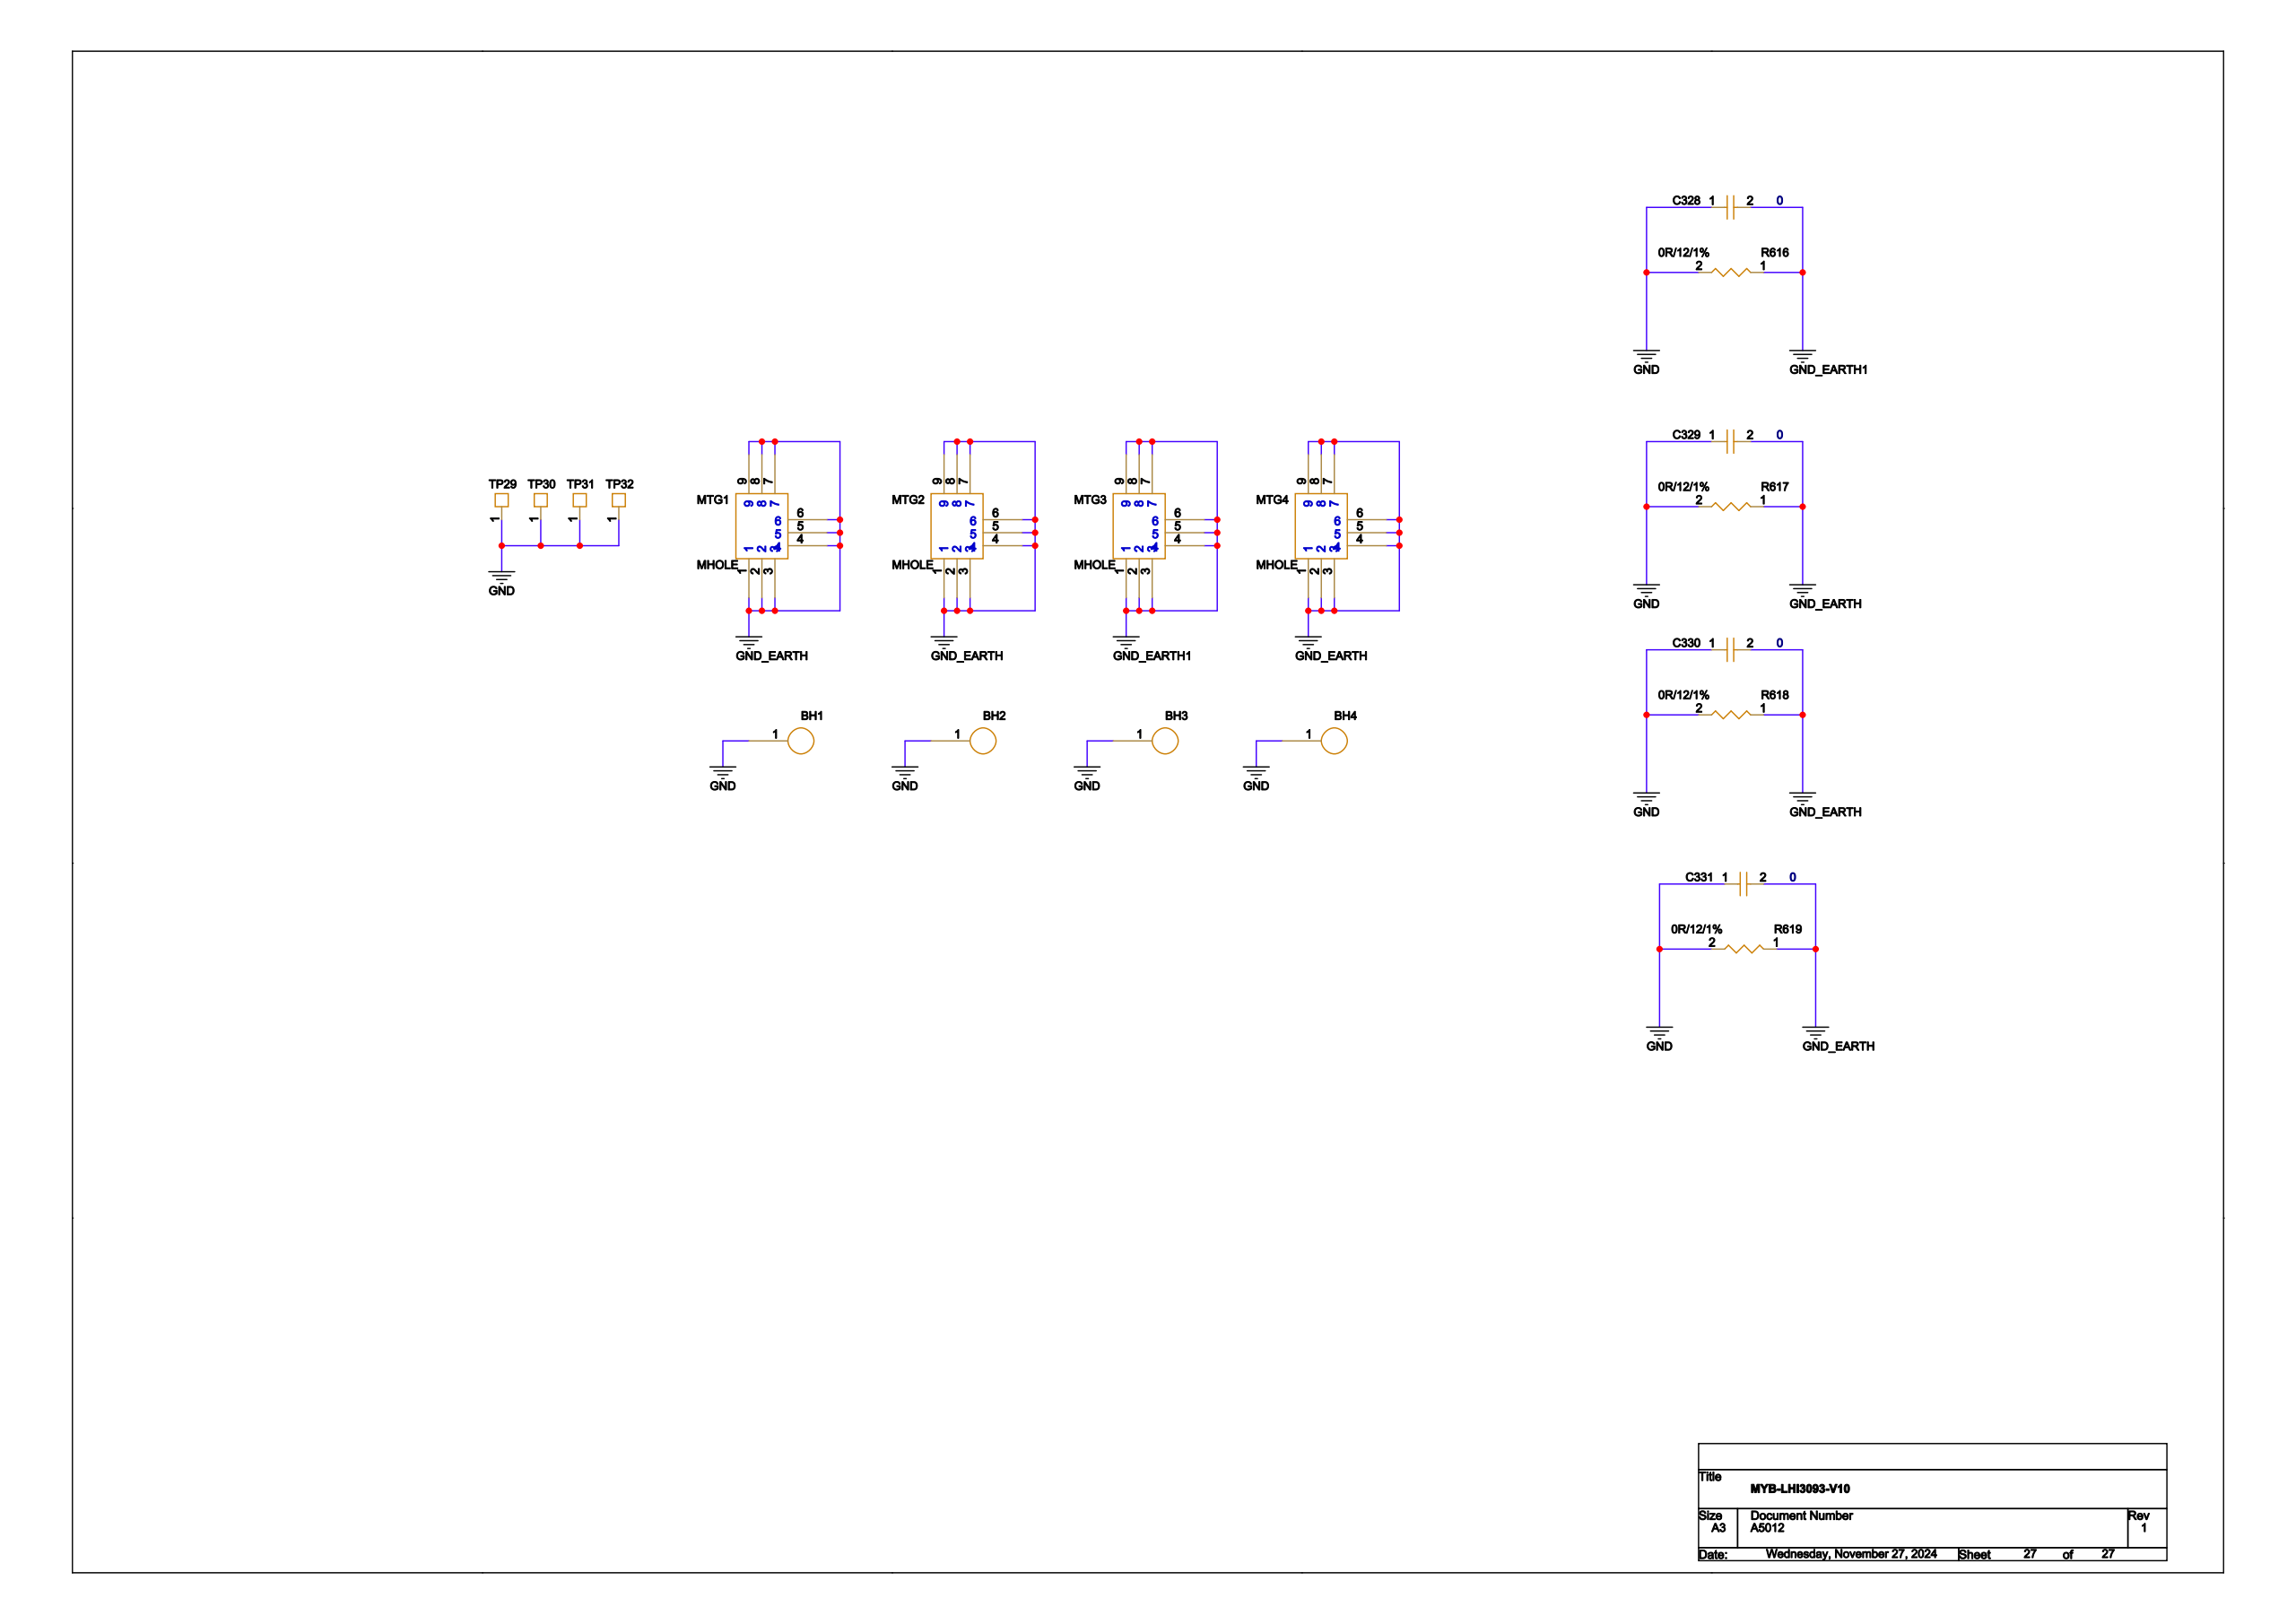Circuit board | Cadence Allegro | 1159 parts | 708 nets | one sheet of the schematic
Parts on this sheet (reference | value | footprint):
BH1 | TP | MH236-125T
BH2 | TP | MH236-125T
BH3 | TP | MH236-125T
BH4 | TP | MH236-125T
C328 | 0 | C1206
C329 | 0 | C1206
C330 | 0 | C1206
C331 | 0 | C1206
MTG1 | MHOLE | HOLE3_2P-8
MTG2 | MHOLE | HOLE3_2P-8
MTG3 | MHOLE | HOLE3_2P-8
MTG4 | MHOLE | HOLE3_2P-8
R616 | 0R/12/1% | R1206
R617 | 0R/12/1% | R1206
R618 | 0R/12/1% | R1206
R619 | 0R/12/1% | R1206
TP29 | T POINT S | HOLE-TP0_9S16
TP30 | T POINT S | HOLE-TP0_9S16
TP31 | T POINT S | HOLE-TP0_9S16
TP32 | T POINT S | HOLE-TP0_9S16
Nets of these parts (net: part-pin ...):
GND: BH1-1 BH2-1 BH3-1 BH4-1 C328-1 C329-1 C330-1 C331-1 R616-2 R617-2 R618-2 R619-2 TP29-1 TP30-1 TP31-1 TP32-1
GND_EARTH: C329-2 C330-2 C331-2 MTG1-1 MTG1-2 MTG1-3 MTG1-4 MTG1-5 MTG1-6 MTG1-7 MTG1-8 MTG1-9 MTG2-1 MTG2-2 MTG2-3 MTG2-4 MTG2-5 MTG2-6 MTG2-7 MTG2-8 MTG2-9 MTG4-1 MTG4-2 MTG4-3 MTG4-4 MTG4-5 MTG4-6 MTG4-7 MTG4-8 MTG4-9 R617-1 R618-1 R619-1
GND_EARTH1: C328-2 MTG3-1 MTG3-2 MTG3-3 MTG3-4 MTG3-5 MTG3-6 MTG3-7 MTG3-8 MTG3-9 R616-1